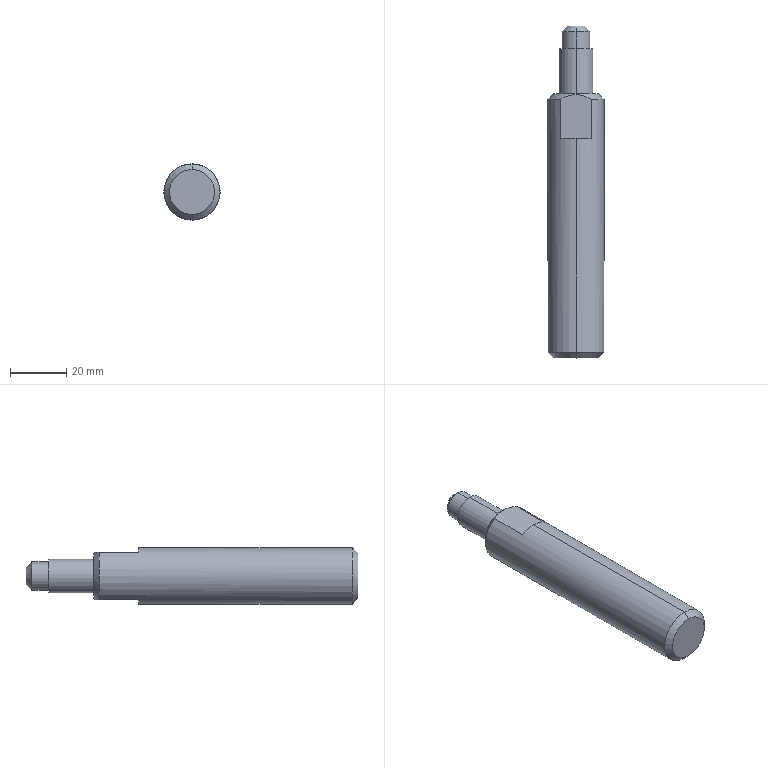Part | STEP file | Foot screw | 1 solid | 20 faces | box 20 x 118 x 20 mm | volume 31335 mm3 | plane 8 | cone 6 | cylinder 6 | commonest cylinder face diameters 10 x2 12 x2 20 x2
STEP:
#1=CARTESIAN_POINT('',(0.,-129.,-8.));
#2=VERTEX_POINT('',#1);
#3=CARTESIAN_POINT('',(0.,-129.,8.));
#4=VERTEX_POINT('',#3);
#5=CARTESIAN_POINT('',(0.,-129.,0.));
#6=DIRECTION('',(0.,-1.,0.));
#7=DIRECTION('',(0.,0.,-1.));
#8=AXIS2_PLACEMENT_3D('',#5,#6,#7);
#9=CIRCLE('',#8,8.);
#10=EDGE_CURVE('',#2,#4,#9,.T.);
#11=ORIENTED_EDGE('',*,*,#10,.F.);
#12=CARTESIAN_POINT('',(0.,-127.,-10.));
#13=VERTEX_POINT('',#12);
#14=CARTESIAN_POINT('',(0.,-127.,-10.));
#15=DIRECTION('',(0.,0.7071,-0.7071));
#16=VECTOR('',#15,1000.);
#17=LINE('',#14,#16);
#18=EDGE_CURVE('',#2,#13,#17,.T.);
#19=ORIENTED_EDGE('',*,*,#18,.T.);
#20=CARTESIAN_POINT('',(0.,-127.,10.));
#21=VERTEX_POINT('',#20);
#22=CARTESIAN_POINT('',(0.,-127.,0.));
#23=DIRECTION('',(0.,1.,0.));
#24=DIRECTION('',(0.,0.,-1.));
#25=AXIS2_PLACEMENT_3D('',#22,#23,#24);
#26=CIRCLE('',#25,10.);
#27=EDGE_CURVE('',#21,#13,#26,.T.);
#28=ORIENTED_EDGE('',*,*,#27,.F.);
#29=CARTESIAN_POINT('',(0.,-127.,10.));
#30=DIRECTION('',(0.,0.7071,0.7071));
#31=VECTOR('',#30,1000.);
#32=LINE('',#29,#31);
#33=EDGE_CURVE('',#4,#21,#32,.T.);
#34=ORIENTED_EDGE('',*,*,#33,.F.);
#35=EDGE_LOOP('',(#11,#19,#28,#34));
#36=FACE_OUTER_BOUND('',#35,.T.);
#37=CARTESIAN_POINT('',(0.,-127.,0.));
#38=DIRECTION('',(0.,1.,0.));
#39=DIRECTION('',(0.,0.,1.));
#40=AXIS2_PLACEMENT_3D('',#37,#38,#39);
#41=CONICAL_SURFACE('',#40,10.,0.7854);
#42=ADVANCED_FACE('',(#36),#41,.T.);
#43=CARTESIAN_POINT('',(0.,-35.,8.));
#44=VERTEX_POINT('',#43);
#45=CARTESIAN_POINT('',(0.,-35.,-8.));
#46=VERTEX_POINT('',#45);
#47=CARTESIAN_POINT('',(0.,-35.,0.));
#48=DIRECTION('',(0.,1.,0.));
#49=DIRECTION('',(0.,0.,1.));
#50=AXIS2_PLACEMENT_3D('',#47,#48,#49);
#51=CIRCLE('',#50,8.);
#52=EDGE_CURVE('',#44,#46,#51,.T.);
#53=ORIENTED_EDGE('',*,*,#52,.F.);
#54=CARTESIAN_POINT('',(0.,-35.4,8.4));
#55=VERTEX_POINT('',#54);
#56=CARTESIAN_POINT('',(0.,-35.,8.));
#57=DIRECTION('',(0.,-0.7071,0.7071));
#58=VECTOR('',#57,1000.);
#59=LINE('',#56,#58);
#60=EDGE_CURVE('',#44,#55,#59,.T.);
#61=ORIENTED_EDGE('',*,*,#60,.T.);
#62=CARTESIAN_POINT('',(5.426,-37.,8.4));
#63=VERTEX_POINT('',#62);
#64=CARTESIAN_POINT('',(5.426,-37.,8.4));
#65=CARTESIAN_POINT('',(5.011,-36.775,8.4));
#66=CARTESIAN_POINT('',(4.587,-36.563,8.4));
#67=CARTESIAN_POINT('',(3.717,-36.177,8.4));
#68=CARTESIAN_POINT('',(3.268,-36.003,8.4));
#69=CARTESIAN_POINT('',(2.359,-35.714,8.4));
#70=CARTESIAN_POINT('',(1.898,-35.599,8.4));
#71=CARTESIAN_POINT('',(0.9592,-35.442,8.4));
#72=CARTESIAN_POINT('',(0.4767,-35.4,8.4));
#73=CARTESIAN_POINT('',(0.,-35.4,8.4));
#74=B_SPLINE_CURVE_WITH_KNOTS('',3,(#64,#65,#66,#67,#68,#69,#70,#71,#72,#73),.UNSPECIFIED.,.F.,.F.,(4,2,2,2,4),(0.005943,0.007357,0.008772,0.01019,0.0116),.UNSPECIFIED.);
#75=EDGE_CURVE('',#63,#55,#74,.T.);
#76=ORIENTED_EDGE('',*,*,#75,.F.);
#77=CARTESIAN_POINT('',(5.426,-37.,-8.4));
#78=VERTEX_POINT('',#77);
#79=CARTESIAN_POINT('',(0.,-37.,0.));
#80=DIRECTION('',(0.,-1.,0.));
#81=DIRECTION('',(0.,0.,1.));
#82=AXIS2_PLACEMENT_3D('',#79,#80,#81);
#83=CIRCLE('',#82,10.);
#84=EDGE_CURVE('',#78,#63,#83,.T.);
#85=ORIENTED_EDGE('',*,*,#84,.F.);
#86=CARTESIAN_POINT('',(0.,-35.4,-8.4));
#87=VERTEX_POINT('',#86);
#88=CARTESIAN_POINT('',(0.,-35.4,-8.4));
#89=CARTESIAN_POINT('',(0.4767,-35.4,-8.4));
#90=CARTESIAN_POINT('',(0.9592,-35.442,-8.4));
#91=CARTESIAN_POINT('',(1.898,-35.599,-8.4));
#92=CARTESIAN_POINT('',(2.359,-35.714,-8.4));
#93=CARTESIAN_POINT('',(3.268,-36.003,-8.4));
#94=CARTESIAN_POINT('',(3.717,-36.177,-8.4));
#95=CARTESIAN_POINT('',(4.587,-36.563,-8.4));
#96=CARTESIAN_POINT('',(5.011,-36.775,-8.4));
#97=CARTESIAN_POINT('',(5.426,-37.,-8.4));
#98=B_SPLINE_CURVE_WITH_KNOTS('',3,(#88,#89,#90,#91,#92,#93,#94,#95,#96,#97),.UNSPECIFIED.,.F.,.F.,(4,2,2,2,4),(0.01936,0.02078,0.0222,0.02362,0.02505),.UNSPECIFIED.);
#99=EDGE_CURVE('',#87,#78,#98,.T.);
#100=ORIENTED_EDGE('',*,*,#99,.F.);
#101=CARTESIAN_POINT('',(0.,-35.,-8.));
#102=DIRECTION('',(0.,-0.7071,-0.7071));
#103=VECTOR('',#102,1000.);
#104=LINE('',#101,#103);
#105=EDGE_CURVE('',#46,#87,#104,.T.);
#106=ORIENTED_EDGE('',*,*,#105,.F.);
#107=EDGE_LOOP('',(#53,#61,#76,#85,#100,#106));
#108=FACE_OUTER_BOUND('',#107,.T.);
#109=CARTESIAN_POINT('',(0.,-35.,0.));
#110=DIRECTION('',(0.,-1.,0.));
#111=DIRECTION('',(0.,0.,-1.));
#112=AXIS2_PLACEMENT_3D('',#109,#110,#111);
#113=CONICAL_SURFACE('',#112,8.,0.7854);
#114=ADVANCED_FACE('',(#108),#113,.T.);
#115=CARTESIAN_POINT('',(0.,-11.,3.));
#116=VERTEX_POINT('',#115);
#117=CARTESIAN_POINT('',(0.,-11.,-3.));
#118=VERTEX_POINT('',#117);
#119=CARTESIAN_POINT('',(0.,-11.,0.));
#120=DIRECTION('',(0.,1.,0.));
#121=DIRECTION('',(0.,0.,1.));
#122=AXIS2_PLACEMENT_3D('',#119,#120,#121);
#123=CIRCLE('',#122,3.);
#124=EDGE_CURVE('',#116,#118,#123,.T.);
#125=ORIENTED_EDGE('',*,*,#124,.F.);
#126=CARTESIAN_POINT('',(0.,-13.,5.));
#127=VERTEX_POINT('',#126);
#128=CARTESIAN_POINT('',(0.,-11.,3.));
#129=DIRECTION('',(0.,-0.7071,0.7071));
#130=VECTOR('',#129,1000.);
#131=LINE('',#128,#130);
#132=EDGE_CURVE('',#116,#127,#131,.T.);
#133=ORIENTED_EDGE('',*,*,#132,.T.);
#134=CARTESIAN_POINT('',(0.,-13.,-5.));
#135=VERTEX_POINT('',#134);
#136=CARTESIAN_POINT('',(0.,-13.,0.));
#137=DIRECTION('',(0.,-1.,0.));
#138=DIRECTION('',(0.,0.,1.));
#139=AXIS2_PLACEMENT_3D('',#136,#137,#138);
#140=CIRCLE('',#139,5.);
#141=EDGE_CURVE('',#135,#127,#140,.T.);
#142=ORIENTED_EDGE('',*,*,#141,.F.);
#143=CARTESIAN_POINT('',(0.,-11.,-3.));
#144=DIRECTION('',(0.,-0.7071,-0.7071));
#145=VECTOR('',#144,1000.);
#146=LINE('',#143,#145);
#147=EDGE_CURVE('',#118,#135,#146,.T.);
#148=ORIENTED_EDGE('',*,*,#147,.F.);
#149=EDGE_LOOP('',(#125,#133,#142,#148));
#150=FACE_OUTER_BOUND('',#149,.T.);
#151=CARTESIAN_POINT('',(0.,-11.,0.));
#152=DIRECTION('',(0.,-1.,0.));
#153=DIRECTION('',(0.,0.,-1.));
#154=AXIS2_PLACEMENT_3D('',#151,#152,#153);
#155=CONICAL_SURFACE('',#154,3.,0.7854);
#156=ADVANCED_FACE('',(#150),#155,.T.);
#157=CARTESIAN_POINT('',(0.,-19.,5.));
#158=VERTEX_POINT('',#157);
#159=CARTESIAN_POINT('',(0.,-19.,-5.));
#160=VERTEX_POINT('',#159);
#161=CARTESIAN_POINT('',(0.,-19.,0.));
#162=DIRECTION('',(0.,1.,0.));
#163=DIRECTION('',(0.,0.,1.));
#164=AXIS2_PLACEMENT_3D('',#161,#162,#163);
#165=CIRCLE('',#164,5.);
#166=EDGE_CURVE('',#158,#160,#165,.T.);
#167=ORIENTED_EDGE('',*,*,#166,.T.);
#168=CARTESIAN_POINT('',(0.,0.,-5.));
#169=DIRECTION('',(0.,1.,0.));
#170=VECTOR('',#169,1000.);
#171=LINE('',#168,#170);
#172=EDGE_CURVE('',#160,#135,#171,.T.);
#173=ORIENTED_EDGE('',*,*,#172,.T.);
#174=ORIENTED_EDGE('',*,*,#141,.T.);
#175=CARTESIAN_POINT('',(0.,0.,5.));
#176=DIRECTION('',(0.,1.,0.));
#177=VECTOR('',#176,1000.);
#178=LINE('',#175,#177);
#179=EDGE_CURVE('',#158,#127,#178,.T.);
#180=ORIENTED_EDGE('',*,*,#179,.F.);
#181=EDGE_LOOP('',(#167,#173,#174,#180));
#182=FACE_OUTER_BOUND('',#181,.T.);
#183=CARTESIAN_POINT('',(0.,0.,0.));
#184=DIRECTION('',(0.,1.,0.));
#185=DIRECTION('',(0.,0.,1.));
#186=AXIS2_PLACEMENT_3D('',#183,#184,#185);
#187=CYLINDRICAL_SURFACE('',#186,5.);
#188=ADVANCED_FACE('',(#182),#187,.T.);
#189=CARTESIAN_POINT('',(0.,-35.,6.));
#190=VERTEX_POINT('',#189);
#191=CARTESIAN_POINT('',(0.,-35.,-6.));
#192=VERTEX_POINT('',#191);
#193=CARTESIAN_POINT('',(0.,-35.,0.));
#194=DIRECTION('',(0.,1.,0.));
#195=DIRECTION('',(0.,0.,1.));
#196=AXIS2_PLACEMENT_3D('',#193,#194,#195);
#197=CIRCLE('',#196,6.);
#198=EDGE_CURVE('',#190,#192,#197,.T.);
#199=ORIENTED_EDGE('',*,*,#198,.T.);
#200=CARTESIAN_POINT('',(0.,-19.,-6.));
#201=VERTEX_POINT('',#200);
#202=CARTESIAN_POINT('',(0.,0.,-6.));
#203=DIRECTION('',(0.,1.,0.));
#204=VECTOR('',#203,1000.);
#205=LINE('',#202,#204);
#206=EDGE_CURVE('',#192,#201,#205,.T.);
#207=ORIENTED_EDGE('',*,*,#206,.T.);
#208=CARTESIAN_POINT('',(0.,-19.,6.));
#209=VERTEX_POINT('',#208);
#210=CARTESIAN_POINT('',(0.,-19.,0.));
#211=DIRECTION('',(0.,1.,0.));
#212=DIRECTION('',(0.,0.,1.));
#213=AXIS2_PLACEMENT_3D('',#210,#211,#212);
#214=CIRCLE('',#213,6.);
#215=EDGE_CURVE('',#209,#201,#214,.T.);
#216=ORIENTED_EDGE('',*,*,#215,.F.);
#217=CARTESIAN_POINT('',(0.,0.,6.));
#218=DIRECTION('',(0.,1.,0.));
#219=VECTOR('',#218,1000.);
#220=LINE('',#217,#219);
#221=EDGE_CURVE('',#190,#209,#220,.T.);
#222=ORIENTED_EDGE('',*,*,#221,.F.);
#223=EDGE_LOOP('',(#199,#207,#216,#222));
#224=FACE_OUTER_BOUND('',#223,.T.);
#225=CARTESIAN_POINT('',(0.,0.,0.));
#226=DIRECTION('',(0.,1.,0.));
#227=DIRECTION('',(0.,0.,1.));
#228=AXIS2_PLACEMENT_3D('',#225,#226,#227);
#229=CYLINDRICAL_SURFACE('',#228,6.);
#230=ADVANCED_FACE('',(#224),#229,.T.);
#231=ORIENTED_EDGE('',*,*,#27,.T.);
#232=CARTESIAN_POINT('',(0.,-51.,-10.));
#233=VERTEX_POINT('',#232);
#234=CARTESIAN_POINT('',(0.,0.,-10.));
#235=DIRECTION('',(0.,1.,0.));
#236=VECTOR('',#235,1000.);
#237=LINE('',#234,#236);
#238=EDGE_CURVE('',#13,#233,#237,.T.);
#239=ORIENTED_EDGE('',*,*,#238,.T.);
#240=CARTESIAN_POINT('',(5.426,-51.,-8.4));
#241=VERTEX_POINT('',#240);
#242=CARTESIAN_POINT('',(0.,-51.,0.));
#243=DIRECTION('',(0.,1.,0.));
#244=DIRECTION('',(0.,0.,-1.));
#245=AXIS2_PLACEMENT_3D('',#242,#243,#244);
#246=CIRCLE('',#245,10.);
#247=EDGE_CURVE('',#241,#233,#246,.T.);
#248=ORIENTED_EDGE('',*,*,#247,.F.);
#249=CARTESIAN_POINT('',(5.426,0.,-8.4));
#250=DIRECTION('',(0.,-1.,0.));
#251=VECTOR('',#250,1000.);
#252=LINE('',#249,#251);
#253=EDGE_CURVE('',#78,#241,#252,.T.);
#254=ORIENTED_EDGE('',*,*,#253,.F.);
#255=ORIENTED_EDGE('',*,*,#84,.T.);
#256=CARTESIAN_POINT('',(5.426,-51.,8.4));
#257=VERTEX_POINT('',#256);
#258=CARTESIAN_POINT('',(5.426,0.,8.4));
#259=DIRECTION('',(0.,1.,0.));
#260=VECTOR('',#259,1000.);
#261=LINE('',#258,#260);
#262=EDGE_CURVE('',#257,#63,#261,.T.);
#263=ORIENTED_EDGE('',*,*,#262,.F.);
#264=CARTESIAN_POINT('',(0.,-51.,10.));
#265=VERTEX_POINT('',#264);
#266=CARTESIAN_POINT('',(0.,-51.,0.));
#267=DIRECTION('',(0.,1.,0.));
#268=DIRECTION('',(0.,0.,-1.));
#269=AXIS2_PLACEMENT_3D('',#266,#267,#268);
#270=CIRCLE('',#269,10.);
#271=EDGE_CURVE('',#265,#257,#270,.T.);
#272=ORIENTED_EDGE('',*,*,#271,.F.);
#273=CARTESIAN_POINT('',(0.,0.,10.));
#274=DIRECTION('',(0.,1.,0.));
#275=VECTOR('',#274,1000.);
#276=LINE('',#273,#275);
#277=EDGE_CURVE('',#21,#265,#276,.T.);
#278=ORIENTED_EDGE('',*,*,#277,.F.);
#279=EDGE_LOOP('',(#231,#239,#248,#254,#255,#263,#272,#278));
#280=FACE_OUTER_BOUND('',#279,.T.);
#281=CARTESIAN_POINT('',(0.,0.,0.));
#282=DIRECTION('',(0.,1.,0.));
#283=DIRECTION('',(0.,0.,1.));
#284=AXIS2_PLACEMENT_3D('',#281,#282,#283);
#285=CYLINDRICAL_SURFACE('',#284,10.);
#286=ADVANCED_FACE('',(#280),#285,.T.);
#287=CARTESIAN_POINT('',(0.,-129.,0.));
#288=DIRECTION('',(0.,-1.,0.));
#289=DIRECTION('',(0.,0.,-1.));
#290=AXIS2_PLACEMENT_3D('',#287,#288,#289);
#291=CIRCLE('',#290,8.);
#292=EDGE_CURVE('',#4,#2,#291,.T.);
#293=ORIENTED_EDGE('',*,*,#292,.T.);
#294=ORIENTED_EDGE('',*,*,#10,.T.);
#295=EDGE_LOOP('',(#293,#294));
#296=FACE_OUTER_BOUND('',#295,.T.);
#297=CARTESIAN_POINT('',(0.,-129.,0.));
#298=DIRECTION('',(0.,-1.,0.));
#299=DIRECTION('',(0.,0.,-1.));
#300=AXIS2_PLACEMENT_3D('',#297,#298,#299);
#301=PLANE('',#300);
#302=ADVANCED_FACE('',(#296),#301,.T.);
#303=ORIENTED_EDGE('',*,*,#238,.F.);
#304=CARTESIAN_POINT('',(0.,-127.,0.));
#305=DIRECTION('',(0.,1.,0.));
#306=DIRECTION('',(0.,0.,-1.));
#307=AXIS2_PLACEMENT_3D('',#304,#305,#306);
#308=CIRCLE('',#307,10.);
#309=EDGE_CURVE('',#13,#21,#308,.T.);
#310=ORIENTED_EDGE('',*,*,#309,.T.);
#311=ORIENTED_EDGE('',*,*,#277,.T.);
#312=CARTESIAN_POINT('',(-5.426,-51.,8.4));
#313=VERTEX_POINT('',#312);
#314=CARTESIAN_POINT('',(0.,-51.,0.));
#315=DIRECTION('',(0.,1.,0.));
#316=DIRECTION('',(0.,0.,-1.));
#317=AXIS2_PLACEMENT_3D('',#314,#315,#316);
#318=CIRCLE('',#317,10.);
#319=EDGE_CURVE('',#313,#265,#318,.T.);
#320=ORIENTED_EDGE('',*,*,#319,.F.);
#321=CARTESIAN_POINT('',(-5.426,-37.,8.4));
#322=VERTEX_POINT('',#321);
#323=CARTESIAN_POINT('',(-5.426,0.,8.4));
#324=DIRECTION('',(0.,-1.,0.));
#325=VECTOR('',#324,1000.);
#326=LINE('',#323,#325);
#327=EDGE_CURVE('',#322,#313,#326,.T.);
#328=ORIENTED_EDGE('',*,*,#327,.F.);
#329=CARTESIAN_POINT('',(-5.426,-37.,-8.4));
#330=VERTEX_POINT('',#329);
#331=CARTESIAN_POINT('',(0.,-37.,0.));
#332=DIRECTION('',(0.,-1.,0.));
#333=DIRECTION('',(0.,0.,1.));
#334=AXIS2_PLACEMENT_3D('',#331,#332,#333);
#335=CIRCLE('',#334,10.);
#336=EDGE_CURVE('',#322,#330,#335,.T.);
#337=ORIENTED_EDGE('',*,*,#336,.T.);
#338=CARTESIAN_POINT('',(-5.426,-51.,-8.4));
#339=VERTEX_POINT('',#338);
#340=CARTESIAN_POINT('',(-5.426,0.,-8.4));
#341=DIRECTION('',(0.,1.,0.));
#342=VECTOR('',#341,1000.);
#343=LINE('',#340,#342);
#344=EDGE_CURVE('',#339,#330,#343,.T.);
#345=ORIENTED_EDGE('',*,*,#344,.F.);
#346=CARTESIAN_POINT('',(0.,-51.,0.));
#347=DIRECTION('',(0.,1.,0.));
#348=DIRECTION('',(0.,0.,-1.));
#349=AXIS2_PLACEMENT_3D('',#346,#347,#348);
#350=CIRCLE('',#349,10.);
#351=EDGE_CURVE('',#233,#339,#350,.T.);
#352=ORIENTED_EDGE('',*,*,#351,.F.);
#353=EDGE_LOOP('',(#303,#310,#311,#320,#328,#337,#345,#352));
#354=FACE_OUTER_BOUND('',#353,.T.);
#355=CARTESIAN_POINT('',(0.,0.,0.));
#356=DIRECTION('',(0.,1.,0.));
#357=DIRECTION('',(0.,0.,1.));
#358=AXIS2_PLACEMENT_3D('',#355,#356,#357);
#359=CYLINDRICAL_SURFACE('',#358,10.);
#360=ADVANCED_FACE('',(#354),#359,.T.);
#361=CARTESIAN_POINT('',(0.,-35.,0.));
#362=DIRECTION('',(0.,1.,0.));
#363=DIRECTION('',(0.,0.,1.));
#364=AXIS2_PLACEMENT_3D('',#361,#362,#363);
#365=CIRCLE('',#364,8.);
#366=EDGE_CURVE('',#46,#44,#365,.T.);
#367=ORIENTED_EDGE('',*,*,#366,.T.);
#368=ORIENTED_EDGE('',*,*,#52,.T.);
#369=EDGE_LOOP('',(#367,#368));
#370=FACE_OUTER_BOUND('',#369,.T.);
#371=ORIENTED_EDGE('',*,*,#198,.F.);
#372=CARTESIAN_POINT('',(0.,-35.,0.));
#373=DIRECTION('',(0.,1.,0.));
#374=DIRECTION('',(0.,0.,1.));
#375=AXIS2_PLACEMENT_3D('',#372,#373,#374);
#376=CIRCLE('',#375,6.);
#377=EDGE_CURVE('',#192,#190,#376,.T.);
#378=ORIENTED_EDGE('',*,*,#377,.F.);
#379=EDGE_LOOP('',(#371,#378));
#380=FACE_BOUND('',#379,.T.);
#381=CARTESIAN_POINT('',(0.,-35.,10.));
#382=DIRECTION('',(0.,1.,0.));
#383=DIRECTION('',(0.,0.,1.));
#384=AXIS2_PLACEMENT_3D('',#381,#382,#383);
#385=PLANE('',#384);
#386=ADVANCED_FACE('',(#370,#380),#385,.T.);
#387=ORIENTED_EDGE('',*,*,#206,.F.);
#388=ORIENTED_EDGE('',*,*,#377,.T.);
#389=ORIENTED_EDGE('',*,*,#221,.T.);
#390=CARTESIAN_POINT('',(0.,-19.,0.));
#391=DIRECTION('',(0.,1.,0.));
#392=DIRECTION('',(0.,0.,1.));
#393=AXIS2_PLACEMENT_3D('',#390,#391,#392);
#394=CIRCLE('',#393,6.);
#395=EDGE_CURVE('',#201,#209,#394,.T.);
#396=ORIENTED_EDGE('',*,*,#395,.F.);
#397=EDGE_LOOP('',(#387,#388,#389,#396));
#398=FACE_OUTER_BOUND('',#397,.T.);
#399=CARTESIAN_POINT('',(0.,0.,0.));
#400=DIRECTION('',(0.,1.,0.));
#401=DIRECTION('',(0.,0.,1.));
#402=AXIS2_PLACEMENT_3D('',#399,#400,#401);
#403=CYLINDRICAL_SURFACE('',#402,6.);
#404=ADVANCED_FACE('',(#398),#403,.T.);
#405=ORIENTED_EDGE('',*,*,#215,.T.);
#406=ORIENTED_EDGE('',*,*,#395,.T.);
#407=EDGE_LOOP('',(#405,#406));
#408=FACE_OUTER_BOUND('',#407,.T.);
#409=ORIENTED_EDGE('',*,*,#166,.F.);
#410=CARTESIAN_POINT('',(0.,-19.,0.));
#411=DIRECTION('',(0.,1.,0.));
#412=DIRECTION('',(0.,0.,1.));
#413=AXIS2_PLACEMENT_3D('',#410,#411,#412);
#414=CIRCLE('',#413,5.);
#415=EDGE_CURVE('',#160,#158,#414,.T.);
#416=ORIENTED_EDGE('',*,*,#415,.F.);
#417=EDGE_LOOP('',(#409,#416));
#418=FACE_BOUND('',#417,.T.);
#419=CARTESIAN_POINT('',(0.,-19.,6.));
#420=DIRECTION('',(0.,1.,0.));
#421=DIRECTION('',(0.,0.,1.));
#422=AXIS2_PLACEMENT_3D('',#419,#420,#421);
#423=PLANE('',#422);
#424=ADVANCED_FACE('',(#408,#418),#423,.T.);
#425=ORIENTED_EDGE('',*,*,#172,.F.);
#426=ORIENTED_EDGE('',*,*,#415,.T.);
#427=ORIENTED_EDGE('',*,*,#179,.T.);
#428=CARTESIAN_POINT('',(0.,-13.,0.));
#429=DIRECTION('',(0.,-1.,0.));
#430=DIRECTION('',(0.,0.,1.));
#431=AXIS2_PLACEMENT_3D('',#428,#429,#430);
#432=CIRCLE('',#431,5.);
#433=EDGE_CURVE('',#127,#135,#432,.T.);
#434=ORIENTED_EDGE('',*,*,#433,.T.);
#435=EDGE_LOOP('',(#425,#426,#427,#434));
#436=FACE_OUTER_BOUND('',#435,.T.);
#437=CARTESIAN_POINT('',(0.,0.,0.));
#438=DIRECTION('',(0.,1.,0.));
#439=DIRECTION('',(0.,0.,1.));
#440=AXIS2_PLACEMENT_3D('',#437,#438,#439);
#441=CYLINDRICAL_SURFACE('',#440,5.);
#442=ADVANCED_FACE('',(#436),#441,.T.);
#443=CARTESIAN_POINT('',(0.,-11.,0.));
#444=DIRECTION('',(0.,1.,0.));
#445=DIRECTION('',(0.,0.,1.));
#446=AXIS2_PLACEMENT_3D('',#443,#444,#445);
#447=CIRCLE('',#446,3.);
#448=EDGE_CURVE('',#118,#116,#447,.T.);
#449=ORIENTED_EDGE('',*,*,#448,.T.);
#450=ORIENTED_EDGE('',*,*,#124,.T.);
#451=EDGE_LOOP('',(#449,#450));
#452=FACE_OUTER_BOUND('',#451,.T.);
#453=CARTESIAN_POINT('',(0.,-11.,5.));
#454=DIRECTION('',(0.,1.,0.));
#455=DIRECTION('',(0.,0.,1.));
#456=AXIS2_PLACEMENT_3D('',#453,#454,#455);
#457=PLANE('',#456);
#458=ADVANCED_FACE('',(#452),#457,.T.);
#459=ORIENTED_EDGE('',*,*,#132,.F.);
#460=ORIENTED_EDGE('',*,*,#448,.F.);
#461=ORIENTED_EDGE('',*,*,#147,.T.);
#462=ORIENTED_EDGE('',*,*,#433,.F.);
#463=EDGE_LOOP('',(#459,#460,#461,#462));
#464=FACE_OUTER_BOUND('',#463,.T.);
#465=CARTESIAN_POINT('',(0.,-11.,0.));
#466=DIRECTION('',(0.,-1.,0.));
#467=DIRECTION('',(0.,0.,-1.));
#468=AXIS2_PLACEMENT_3D('',#465,#466,#467);
#469=CONICAL_SURFACE('',#468,3.,0.7854);
#470=ADVANCED_FACE('',(#464),#469,.T.);
#471=ORIENTED_EDGE('',*,*,#60,.F.);
#472=ORIENTED_EDGE('',*,*,#366,.F.);
#473=ORIENTED_EDGE('',*,*,#105,.T.);
#474=CARTESIAN_POINT('',(-5.426,-37.,-8.4));
#475=CARTESIAN_POINT('',(-4.589,-36.546,-8.4));
#476=CARTESIAN_POINT('',(-3.726,-36.148,-8.4));
#477=CARTESIAN_POINT('',(-2.357,-35.714,-8.4));
#478=CARTESIAN_POINT('',(-1.889,-35.597,-8.4));
#479=CARTESIAN_POINT('',(-0.9507,-35.441,-8.4));
#480=CARTESIAN_POINT('',(-0.4775,-35.4,-8.4));
#481=CARTESIAN_POINT('',(0.,-35.4,-8.4));
#482=B_SPLINE_CURVE_WITH_KNOTS('',3,(#474,#475,#476,#477,#478,#479,#480,#481),.UNSPECIFIED.,.F.,.F.,(4,2,2,4),(0.01366,0.01651,0.01793,0.01936),.UNSPECIFIED.);
#483=EDGE_CURVE('',#330,#87,#482,.T.);
#484=ORIENTED_EDGE('',*,*,#483,.F.);
#485=ORIENTED_EDGE('',*,*,#336,.F.);
#486=CARTESIAN_POINT('',(0.,-35.4,8.4));
#487=CARTESIAN_POINT('',(-0.4775,-35.4,8.4));
#488=CARTESIAN_POINT('',(-0.9507,-35.441,8.4));
#489=CARTESIAN_POINT('',(-1.889,-35.597,8.4));
#490=CARTESIAN_POINT('',(-2.357,-35.714,8.4));
#491=CARTESIAN_POINT('',(-3.726,-36.148,8.4));
#492=CARTESIAN_POINT('',(-4.589,-36.546,8.4));
#493=CARTESIAN_POINT('',(-5.426,-37.,8.4));
#494=B_SPLINE_CURVE_WITH_KNOTS('',3,(#486,#487,#488,#489,#490,#491,#492,#493),.UNSPECIFIED.,.F.,.F.,(4,2,2,4),(0.0116,0.01302,0.01444,0.01727),.UNSPECIFIED.);
#495=EDGE_CURVE('',#55,#322,#494,.T.);
#496=ORIENTED_EDGE('',*,*,#495,.F.);
#497=EDGE_LOOP('',(#471,#472,#473,#484,#485,#496));
#498=FACE_OUTER_BOUND('',#497,.T.);
#499=CARTESIAN_POINT('',(0.,-35.,0.));
#500=DIRECTION('',(0.,-1.,0.));
#501=DIRECTION('',(0.,0.,-1.));
#502=AXIS2_PLACEMENT_3D('',#499,#500,#501);
#503=CONICAL_SURFACE('',#502,8.,0.7854);
#504=ADVANCED_FACE('',(#498),#503,.T.);
#505=ORIENTED_EDGE('',*,*,#18,.F.);
#506=ORIENTED_EDGE('',*,*,#292,.F.);
#507=ORIENTED_EDGE('',*,*,#33,.T.);
#508=ORIENTED_EDGE('',*,*,#309,.F.);
#509=EDGE_LOOP('',(#505,#506,#507,#508));
#510=FACE_OUTER_BOUND('',#509,.T.);
#511=CARTESIAN_POINT('',(0.,-127.,0.));
#512=DIRECTION('',(0.,1.,0.));
#513=DIRECTION('',(0.,0.,1.));
#514=AXIS2_PLACEMENT_3D('',#511,#512,#513);
#515=CONICAL_SURFACE('',#514,10.,0.7854);
#516=ADVANCED_FACE('',(#510),#515,.T.);
#517=CARTESIAN_POINT('',(-10.,-51.,8.4));
#518=DIRECTION('',(1.,0.,0.));
#519=VECTOR('',#518,1000.);
#520=LINE('',#517,#519);
#521=EDGE_CURVE('',#313,#257,#520,.T.);
#522=ORIENTED_EDGE('',*,*,#521,.F.);
#523=ORIENTED_EDGE('',*,*,#319,.T.);
#524=ORIENTED_EDGE('',*,*,#271,.T.);
#525=EDGE_LOOP('',(#522,#523,#524));
#526=FACE_OUTER_BOUND('',#525,.T.);
#527=CARTESIAN_POINT('',(-10.,-51.,8.4));
#528=DIRECTION('',(0.,-1.,0.));
#529=DIRECTION('',(0.,0.,-1.));
#530=AXIS2_PLACEMENT_3D('',#527,#528,#529);
#531=PLANE('',#530);
#532=ADVANCED_FACE('',(#526),#531,.F.);
#533=ORIENTED_EDGE('',*,*,#327,.T.);
#534=ORIENTED_EDGE('',*,*,#521,.T.);
#535=ORIENTED_EDGE('',*,*,#262,.T.);
#536=ORIENTED_EDGE('',*,*,#75,.T.);
#537=ORIENTED_EDGE('',*,*,#495,.T.);
#538=EDGE_LOOP('',(#533,#534,#535,#536,#537));
#539=FACE_OUTER_BOUND('',#538,.T.);
#540=CARTESIAN_POINT('',(-10.,-35.,8.4));
#541=DIRECTION('',(0.,0.,-1.));
#542=DIRECTION('',(0.,1.,0.));
#543=AXIS2_PLACEMENT_3D('',#540,#541,#542);
#544=PLANE('',#543);
#545=ADVANCED_FACE('',(#539),#544,.F.);
#546=ORIENTED_EDGE('',*,*,#253,.T.);
#547=CARTESIAN_POINT('',(-10.,-51.,-8.4));
#548=DIRECTION('',(1.,0.,0.));
#549=VECTOR('',#548,1000.);
#550=LINE('',#547,#549);
#551=EDGE_CURVE('',#339,#241,#550,.T.);
#552=ORIENTED_EDGE('',*,*,#551,.F.);
#553=ORIENTED_EDGE('',*,*,#344,.T.);
#554=ORIENTED_EDGE('',*,*,#483,.T.);
#555=ORIENTED_EDGE('',*,*,#99,.T.);
#556=EDGE_LOOP('',(#546,#552,#553,#554,#555));
#557=FACE_OUTER_BOUND('',#556,.T.);
#558=CARTESIAN_POINT('',(-10.,-35.,-8.4));
#559=DIRECTION('',(0.,0.,1.));
#560=DIRECTION('',(0.,-1.,0.));
#561=AXIS2_PLACEMENT_3D('',#558,#559,#560);
#562=PLANE('',#561);
#563=ADVANCED_FACE('',(#557),#562,.F.);
#564=ORIENTED_EDGE('',*,*,#247,.T.);
#565=ORIENTED_EDGE('',*,*,#351,.T.);
#566=ORIENTED_EDGE('',*,*,#551,.T.);
#567=EDGE_LOOP('',(#564,#565,#566));
#568=FACE_OUTER_BOUND('',#567,.T.);
#569=CARTESIAN_POINT('',(-10.,-51.,-8.4));
#570=DIRECTION('',(0.,-1.,0.));
#571=DIRECTION('',(0.,0.,-1.));
#572=AXIS2_PLACEMENT_3D('',#569,#570,#571);
#573=PLANE('',#572);
#574=ADVANCED_FACE('',(#568),#573,.F.);
#575=CLOSED_SHELL('',(#42,#114,#156,#188,#230,#286,#302,#360,#386,#404,#424,#442,#458,#470,#504,#516,#532,#545,#563,#574));
#576=MANIFOLD_SOLID_BREP('',#575);
#577=CARTESIAN_POINT('',(0.,0.,0.));
#578=DIRECTION('',(0.,0.,1.));
#579=DIRECTION('',(1.,0.,0.));
#580=AXIS2_PLACEMENT_3D('',#577,#578,#579);
#581=(LENGTH_UNIT()NAMED_UNIT(*)SI_UNIT(.MILLI.,.METRE.));
#582=UNCERTAINTY_MEASURE_WITH_UNIT(LENGTH_MEASURE(0.00001),#581,'','');
#583=(NAMED_UNIT(*)PLANE_ANGLE_UNIT()SI_UNIT($,.RADIAN.));
#584=(NAMED_UNIT(*)SI_UNIT($,.STERADIAN.)SOLID_ANGLE_UNIT());
#585=(GEOMETRIC_REPRESENTATION_CONTEXT(3)GLOBAL_UNCERTAINTY_ASSIGNED_CONTEXT((#582))GLOBAL_UNIT_ASSIGNED_CONTEXT((#581,#583,#584))REPRESENTATION_CONTEXT('',''));
#586=ADVANCED_BREP_SHAPE_REPRESENTATION('',(#576,#580),#585);